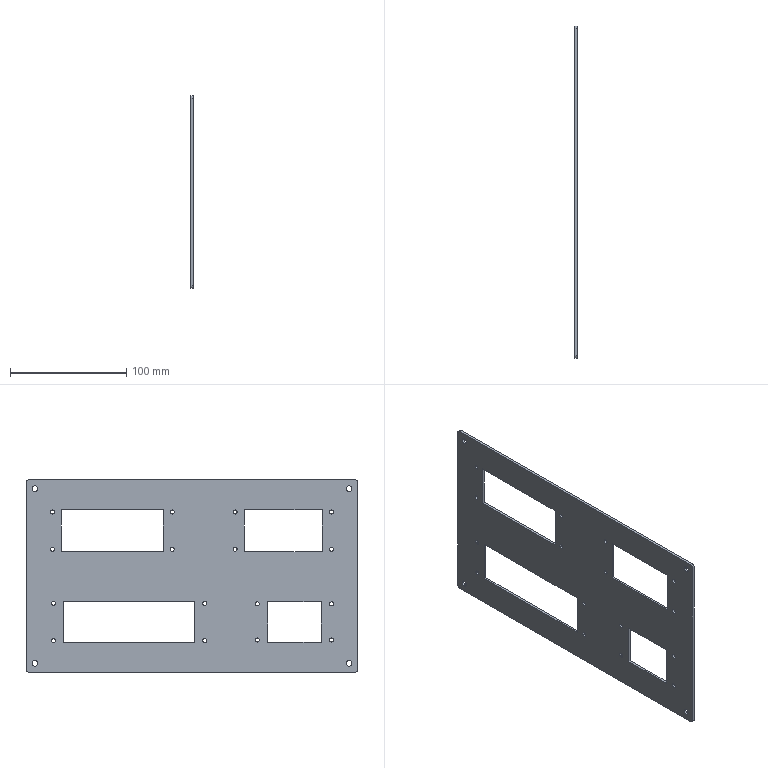Part | NX | features solid 2 | 1 solid | 66 faces | box 2 x 285 x 165 mm | volume 71069 mm3 | cylinder 44 | plane 22 | commonest cylinder face diameters 3.459 x32 5 x8 4 x4